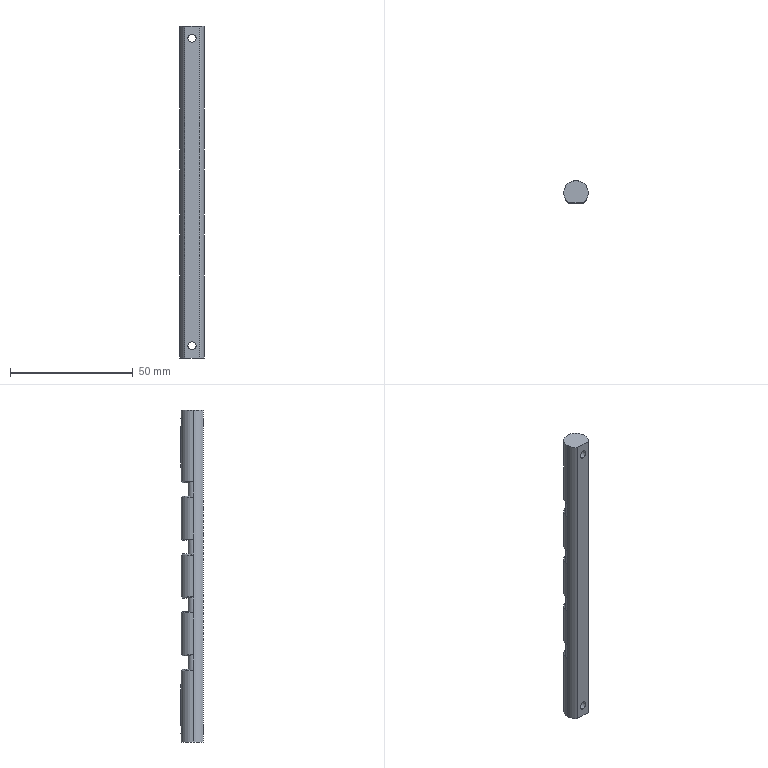Part | SolidWorks | features ICE 3, Chamfer 1, Extrusion 1, Fillet 1, HoleWzd 1 | 1 solid | 42 faces | box 10 x 9 x 135 mm | volume 9423 mm3 | cylinder 19 | plane 15 | cone 8 | commonest cylinder face diameters 4 x8 10 x7 3.3 x4